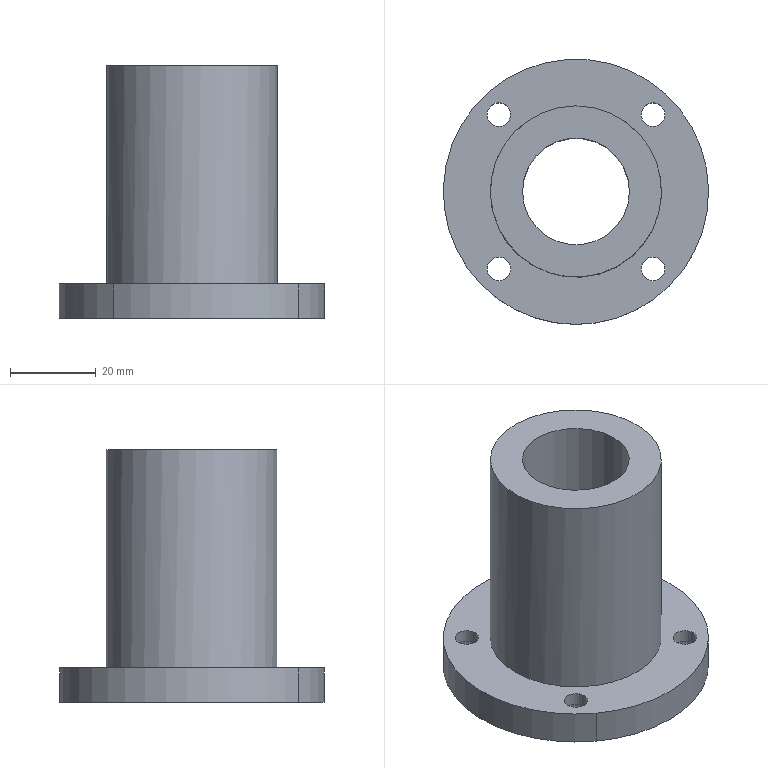Part | STEP file | YBQDJ-QD-7 | 1 solid | 19 faces | box 62 x 62 x 59 mm | volume 57722 mm3 | cylinder 12 | plane 7 | commonest cylinder face diameters 5.5 x4 9 x4 62 x2 25 x1 40 x1
STEP:
#1=CARTESIAN_POINT('',(0.,0.,0.));
#2=DIRECTION('',(0.,0.,1.));
#3=DIRECTION('',(1.,0.,0.));
#4=AXIS2_PLACEMENT_3D('',#1,#2,#3);
#5=CARTESIAN_POINT('',(-327.5,-310.,166.));
#6=VERTEX_POINT('',#5);
#7=CARTESIAN_POINT('',(-340.,-310.,166.));
#8=DIRECTION('',(0.,0.,-1.));
#9=DIRECTION('',(1.,0.,0.));
#10=AXIS2_PLACEMENT_3D('',#7,#8,#9);
#11=CIRCLE('',#10,12.5);
#12=CARTESIAN_POINT('',(-340.,-310.,166.));
#13=DIRECTION('',(0.,0.,-1.));
#14=DIRECTION('',(1.,0.,0.));
#15=AXIS2_PLACEMENT_3D('',#12,#13,#14);
#16=PLANE('',#15);
#17=CARTESIAN_POINT('',(0.,0.));
#18=DIRECTION('',(1.,0.));
#19=AXIS2_PLACEMENT_2D('',#17,#18);
#20=CIRCLE('',#19,12.5);
#21=(GEOMETRIC_REPRESENTATION_CONTEXT(2)PARAMETRIC_REPRESENTATION_CONTEXT()REPRESENTATION_CONTEXT('',''));
#22=DEFINITIONAL_REPRESENTATION('',(#20),#21);
#23=PCURVE('',#16,#22);
#24=CARTESIAN_POINT('',(-340.,-310.,225.));
#25=DIRECTION('',(0.,0.,-1.));
#26=DIRECTION('',(1.,0.,0.));
#27=AXIS2_PLACEMENT_3D('',#24,#25,#26);
#28=CYLINDRICAL_SURFACE('',#27,12.5);
#29=CARTESIAN_POINT('',(0.,59.));
#30=DIRECTION('',(1.,0.));
#31=VECTOR('',#30,1.);
#32=LINE('',#29,#31);
#33=(GEOMETRIC_REPRESENTATION_CONTEXT(2)PARAMETRIC_REPRESENTATION_CONTEXT()REPRESENTATION_CONTEXT('',''));
#34=DEFINITIONAL_REPRESENTATION('',(#32),#33);
#35=PCURVE('',#28,#34);
#36=SURFACE_CURVE('',#11,(#23,#35),.PCURVE_S1.);
#37=EDGE_CURVE('',#6,#6,#36,.T.);
#38=ORIENTED_EDGE('',*,*,#37,.F.);
#39=EDGE_LOOP('',(#38));
#40=FACE_BOUND('',#39,.T.);
#41=CARTESIAN_POINT('',(-326.469,-328.031,166.));
#42=VERTEX_POINT('',#41);
#43=CARTESIAN_POINT('',(-321.969,-328.031,166.));
#44=DIRECTION('',(0.,0.,1.));
#45=DIRECTION('',(-1.,0.,0.));
#46=AXIS2_PLACEMENT_3D('',#43,#44,#45);
#47=CIRCLE('',#46,4.5);
#48=CARTESIAN_POINT('',(13.531,18.031));
#49=CARTESIAN_POINT('',(13.531,25.825));
#50=CARTESIAN_POINT('',(20.281,21.928));
#51=CARTESIAN_POINT('',(27.031,18.031));
#52=CARTESIAN_POINT('',(20.281,14.134));
#53=CARTESIAN_POINT('',(13.531,10.237));
#54=CARTESIAN_POINT('',(13.531,18.031));
#55=(BOUNDED_CURVE()B_SPLINE_CURVE(2,(#48,#49,#50,#51,#52,#53,#54),.UNSPECIFIED.,.T.,.F.)B_SPLINE_CURVE_WITH_KNOTS((1,2,2,2,2,1),(-2.094,0.,2.094,4.189,6.283,8.378),.UNSPECIFIED.)CURVE()GEOMETRIC_REPRESENTATION_ITEM()RATIONAL_B_SPLINE_CURVE((1.,0.5,1.,0.5,1.,0.5,1.))REPRESENTATION_ITEM(''));
#56=(GEOMETRIC_REPRESENTATION_CONTEXT(2)PARAMETRIC_REPRESENTATION_CONTEXT()REPRESENTATION_CONTEXT('',''));
#57=DEFINITIONAL_REPRESENTATION('',(#55),#56);
#58=PCURVE('',#16,#57);
#59=CARTESIAN_POINT('',(-321.969,-328.031,166.));
#60=DIRECTION('',(0.,0.,1.));
#61=DIRECTION('',(-1.,0.,0.));
#62=AXIS2_PLACEMENT_3D('',#59,#60,#61);
#63=CYLINDRICAL_SURFACE('',#62,4.5);
#64=CARTESIAN_POINT('',(0.,0.));
#65=DIRECTION('',(1.,0.));
#66=VECTOR('',#65,1.);
#67=LINE('',#64,#66);
#68=(GEOMETRIC_REPRESENTATION_CONTEXT(2)PARAMETRIC_REPRESENTATION_CONTEXT()REPRESENTATION_CONTEXT('',''));
#69=DEFINITIONAL_REPRESENTATION('',(#67),#68);
#70=PCURVE('',#63,#69);
#71=SURFACE_CURVE('',#47,(#58,#70),.PCURVE_S1.);
#72=EDGE_CURVE('',#42,#42,#71,.T.);
#73=ORIENTED_EDGE('',*,*,#72,.T.);
#74=EDGE_LOOP('',(#73));
#75=FACE_BOUND('',#74,.T.);
#76=CARTESIAN_POINT('',(-362.531,-328.031,166.));
#77=VERTEX_POINT('',#76);
#78=CARTESIAN_POINT('',(-358.031,-328.031,166.));
#79=DIRECTION('',(0.,0.,1.));
#80=DIRECTION('',(-1.,0.,0.));
#81=AXIS2_PLACEMENT_3D('',#78,#79,#80);
#82=CIRCLE('',#81,4.5);
#83=CARTESIAN_POINT('',(-22.531,18.031));
#84=CARTESIAN_POINT('',(-22.531,25.825));
#85=CARTESIAN_POINT('',(-15.781,21.928));
#86=CARTESIAN_POINT('',(-9.031,18.031));
#87=CARTESIAN_POINT('',(-15.781,14.134));
#88=CARTESIAN_POINT('',(-22.531,10.237));
#89=CARTESIAN_POINT('',(-22.531,18.031));
#90=(BOUNDED_CURVE()B_SPLINE_CURVE(2,(#83,#84,#85,#86,#87,#88,#89),.UNSPECIFIED.,.T.,.F.)B_SPLINE_CURVE_WITH_KNOTS((1,2,2,2,2,1),(-2.094,0.,2.094,4.189,6.283,8.378),.UNSPECIFIED.)CURVE()GEOMETRIC_REPRESENTATION_ITEM()RATIONAL_B_SPLINE_CURVE((1.,0.5,1.,0.5,1.,0.5,1.))REPRESENTATION_ITEM(''));
#91=(GEOMETRIC_REPRESENTATION_CONTEXT(2)PARAMETRIC_REPRESENTATION_CONTEXT()REPRESENTATION_CONTEXT('',''));
#92=DEFINITIONAL_REPRESENTATION('',(#90),#91);
#93=PCURVE('',#16,#92);
#94=CARTESIAN_POINT('',(-358.031,-328.031,166.));
#95=DIRECTION('',(0.,0.,1.));
#96=DIRECTION('',(-1.,0.,0.));
#97=AXIS2_PLACEMENT_3D('',#94,#95,#96);
#98=CYLINDRICAL_SURFACE('',#97,4.5);
#99=CARTESIAN_POINT('',(0.,0.));
#100=DIRECTION('',(1.,0.));
#101=VECTOR('',#100,1.);
#102=LINE('',#99,#101);
#103=(GEOMETRIC_REPRESENTATION_CONTEXT(2)PARAMETRIC_REPRESENTATION_CONTEXT()REPRESENTATION_CONTEXT('',''));
#104=DEFINITIONAL_REPRESENTATION('',(#102),#103);
#105=PCURVE('',#98,#104);
#106=SURFACE_CURVE('',#82,(#93,#105),.PCURVE_S1.);
#107=EDGE_CURVE('',#77,#77,#106,.T.);
#108=ORIENTED_EDGE('',*,*,#107,.T.);
#109=EDGE_LOOP('',(#108));
#110=FACE_BOUND('',#109,.T.);
#111=CARTESIAN_POINT('',(-362.531,-291.969,166.));
#112=VERTEX_POINT('',#111);
#113=CARTESIAN_POINT('',(-358.031,-291.969,166.));
#114=DIRECTION('',(0.,0.,1.));
#115=DIRECTION('',(-1.,0.,0.));
#116=AXIS2_PLACEMENT_3D('',#113,#114,#115);
#117=CIRCLE('',#116,4.5);
#118=CARTESIAN_POINT('',(-22.531,-18.031));
#119=CARTESIAN_POINT('',(-22.531,-10.237));
#120=CARTESIAN_POINT('',(-15.781,-14.134));
#121=CARTESIAN_POINT('',(-9.031,-18.031));
#122=CARTESIAN_POINT('',(-15.781,-21.928));
#123=CARTESIAN_POINT('',(-22.531,-25.825));
#124=CARTESIAN_POINT('',(-22.531,-18.031));
#125=(BOUNDED_CURVE()B_SPLINE_CURVE(2,(#118,#119,#120,#121,#122,#123,#124),.UNSPECIFIED.,.T.,.F.)B_SPLINE_CURVE_WITH_KNOTS((1,2,2,2,2,1),(-2.094,0.,2.094,4.189,6.283,8.378),.UNSPECIFIED.)CURVE()GEOMETRIC_REPRESENTATION_ITEM()RATIONAL_B_SPLINE_CURVE((1.,0.5,1.,0.5,1.,0.5,1.))REPRESENTATION_ITEM(''));
#126=(GEOMETRIC_REPRESENTATION_CONTEXT(2)PARAMETRIC_REPRESENTATION_CONTEXT()REPRESENTATION_CONTEXT('',''));
#127=DEFINITIONAL_REPRESENTATION('',(#125),#126);
#128=PCURVE('',#16,#127);
#129=CARTESIAN_POINT('',(-358.031,-291.969,166.));
#130=DIRECTION('',(0.,0.,1.));
#131=DIRECTION('',(-1.,0.,0.));
#132=AXIS2_PLACEMENT_3D('',#129,#130,#131);
#133=CYLINDRICAL_SURFACE('',#132,4.5);
#134=CARTESIAN_POINT('',(0.,0.));
#135=DIRECTION('',(1.,0.));
#136=VECTOR('',#135,1.);
#137=LINE('',#134,#136);
#138=(GEOMETRIC_REPRESENTATION_CONTEXT(2)PARAMETRIC_REPRESENTATION_CONTEXT()REPRESENTATION_CONTEXT('',''));
#139=DEFINITIONAL_REPRESENTATION('',(#137),#138);
#140=PCURVE('',#133,#139);
#141=SURFACE_CURVE('',#117,(#128,#140),.PCURVE_S1.);
#142=EDGE_CURVE('',#112,#112,#141,.T.);
#143=ORIENTED_EDGE('',*,*,#142,.T.);
#144=EDGE_LOOP('',(#143));
#145=FACE_BOUND('',#144,.T.);
#146=CARTESIAN_POINT('',(-326.469,-291.969,166.));
#147=VERTEX_POINT('',#146);
#148=CARTESIAN_POINT('',(-321.969,-291.969,166.));
#149=DIRECTION('',(0.,0.,1.));
#150=DIRECTION('',(-1.,0.,0.));
#151=AXIS2_PLACEMENT_3D('',#148,#149,#150);
#152=CIRCLE('',#151,4.5);
#153=CARTESIAN_POINT('',(13.531,-18.031));
#154=CARTESIAN_POINT('',(13.531,-10.237));
#155=CARTESIAN_POINT('',(20.281,-14.134));
#156=CARTESIAN_POINT('',(27.031,-18.031));
#157=CARTESIAN_POINT('',(20.281,-21.928));
#158=CARTESIAN_POINT('',(13.531,-25.825));
#159=CARTESIAN_POINT('',(13.531,-18.031));
#160=(BOUNDED_CURVE()B_SPLINE_CURVE(2,(#153,#154,#155,#156,#157,#158,#159),.UNSPECIFIED.,.T.,.F.)B_SPLINE_CURVE_WITH_KNOTS((1,2,2,2,2,1),(-2.094,0.,2.094,4.189,6.283,8.378),.UNSPECIFIED.)CURVE()GEOMETRIC_REPRESENTATION_ITEM()RATIONAL_B_SPLINE_CURVE((1.,0.5,1.,0.5,1.,0.5,1.))REPRESENTATION_ITEM(''));
#161=(GEOMETRIC_REPRESENTATION_CONTEXT(2)PARAMETRIC_REPRESENTATION_CONTEXT()REPRESENTATION_CONTEXT('',''));
#162=DEFINITIONAL_REPRESENTATION('',(#160),#161);
#163=PCURVE('',#16,#162);
#164=CARTESIAN_POINT('',(-321.969,-291.969,166.));
#165=DIRECTION('',(0.,0.,1.));
#166=DIRECTION('',(-1.,0.,0.));
#167=AXIS2_PLACEMENT_3D('',#164,#165,#166);
#168=CYLINDRICAL_SURFACE('',#167,4.5);
#169=CARTESIAN_POINT('',(0.,0.));
#170=DIRECTION('',(1.,0.));
#171=VECTOR('',#170,1.);
#172=LINE('',#169,#171);
#173=(GEOMETRIC_REPRESENTATION_CONTEXT(2)PARAMETRIC_REPRESENTATION_CONTEXT()REPRESENTATION_CONTEXT('',''));
#174=DEFINITIONAL_REPRESENTATION('',(#172),#173);
#175=PCURVE('',#168,#174);
#176=SURFACE_CURVE('',#152,(#163,#175),.PCURVE_S1.);
#177=EDGE_CURVE('',#147,#147,#176,.T.);
#178=ORIENTED_EDGE('',*,*,#177,.T.);
#179=EDGE_LOOP('',(#178));
#180=FACE_BOUND('',#179,.T.);
#181=CARTESIAN_POINT('',(-315.,-328.33,166.));
#182=VERTEX_POINT('',#181);
#183=CARTESIAN_POINT('',(-358.33,-335.,166.));
#184=VERTEX_POINT('',#183);
#185=CARTESIAN_POINT('',(-340.,-310.,166.));
#186=DIRECTION('',(0.,0.,1.));
#187=DIRECTION('',(1.,0.,0.));
#188=AXIS2_PLACEMENT_3D('',#185,#186,#187);
#189=CIRCLE('',#188,31.);
#190=CARTESIAN_POINT('',(31.,0.));
#191=CARTESIAN_POINT('',(31.,-53.694));
#192=CARTESIAN_POINT('',(-15.5,-26.847));
#193=CARTESIAN_POINT('',(-62.,0.));
#194=CARTESIAN_POINT('',(-15.5,26.847));
#195=CARTESIAN_POINT('',(31.,53.694));
#196=CARTESIAN_POINT('',(31.,0.));
#197=(BOUNDED_CURVE()B_SPLINE_CURVE(2,(#190,#191,#192,#193,#194,#195,#196),.UNSPECIFIED.,.T.,.F.)B_SPLINE_CURVE_WITH_KNOTS((1,2,2,2,2,1),(-2.094,0.,2.094,4.189,6.283,8.378),.UNSPECIFIED.)CURVE()GEOMETRIC_REPRESENTATION_ITEM()RATIONAL_B_SPLINE_CURVE((1.,0.5,1.,0.5,1.,0.5,1.))REPRESENTATION_ITEM(''));
#198=(GEOMETRIC_REPRESENTATION_CONTEXT(2)PARAMETRIC_REPRESENTATION_CONTEXT()REPRESENTATION_CONTEXT('',''));
#199=DEFINITIONAL_REPRESENTATION('',(#197),#198);
#200=PCURVE('',#16,#199);
#201=CARTESIAN_POINT('',(-340.,-310.,174.));
#202=DIRECTION('',(0.,0.,-1.));
#203=DIRECTION('',(1.,0.,0.));
#204=AXIS2_PLACEMENT_3D('',#201,#202,#203);
#205=CYLINDRICAL_SURFACE('',#204,31.);
#206=CARTESIAN_POINT('',(12.566,8.));
#207=DIRECTION('',(-1.,0.));
#208=VECTOR('',#207,1.);
#209=LINE('',#206,#208);
#210=(GEOMETRIC_REPRESENTATION_CONTEXT(2)PARAMETRIC_REPRESENTATION_CONTEXT()REPRESENTATION_CONTEXT('',''));
#211=DEFINITIONAL_REPRESENTATION('',(#209),#210);
#212=PCURVE('',#205,#211);
#213=SURFACE_CURVE('',#189,(#200,#212),.PCURVE_S1.);
#214=EDGE_CURVE('',#182,#184,#213,.T.);
#215=ORIENTED_EDGE('',*,*,#214,.F.);
#216=CARTESIAN_POINT('',(-340.,-310.,166.));
#217=DIRECTION('',(0.,0.,1.));
#218=DIRECTION('',(1.,0.,0.));
#219=AXIS2_PLACEMENT_3D('',#216,#217,#218);
#220=CIRCLE('',#219,31.);
#221=CARTESIAN_POINT('',(31.,0.));
#222=CARTESIAN_POINT('',(31.,-53.694));
#223=CARTESIAN_POINT('',(-15.5,-26.847));
#224=CARTESIAN_POINT('',(-62.,0.));
#225=CARTESIAN_POINT('',(-15.5,26.847));
#226=CARTESIAN_POINT('',(31.,53.694));
#227=CARTESIAN_POINT('',(31.,0.));
#228=(BOUNDED_CURVE()B_SPLINE_CURVE(2,(#221,#222,#223,#224,#225,#226,#227),.UNSPECIFIED.,.T.,.F.)B_SPLINE_CURVE_WITH_KNOTS((1,2,2,2,2,1),(-2.094,0.,2.094,4.189,6.283,8.378),.UNSPECIFIED.)CURVE()GEOMETRIC_REPRESENTATION_ITEM()RATIONAL_B_SPLINE_CURVE((1.,0.5,1.,0.5,1.,0.5,1.))REPRESENTATION_ITEM(''));
#229=(GEOMETRIC_REPRESENTATION_CONTEXT(2)PARAMETRIC_REPRESENTATION_CONTEXT()REPRESENTATION_CONTEXT('',''));
#230=DEFINITIONAL_REPRESENTATION('',(#228),#229);
#231=PCURVE('',#16,#230);
#232=CARTESIAN_POINT('',(-340.,-310.,174.));
#233=DIRECTION('',(0.,0.,-1.));
#234=DIRECTION('',(1.,0.,0.));
#235=AXIS2_PLACEMENT_3D('',#232,#233,#234);
#236=CYLINDRICAL_SURFACE('',#235,31.);
#237=CARTESIAN_POINT('',(6.283,8.));
#238=DIRECTION('',(-1.,0.));
#239=VECTOR('',#238,1.);
#240=LINE('',#237,#239);
#241=(GEOMETRIC_REPRESENTATION_CONTEXT(2)PARAMETRIC_REPRESENTATION_CONTEXT()REPRESENTATION_CONTEXT('',''));
#242=DEFINITIONAL_REPRESENTATION('',(#240),#241);
#243=PCURVE('',#236,#242);
#244=SURFACE_CURVE('',#220,(#231,#243),.PCURVE_S1.);
#245=EDGE_CURVE('',#184,#182,#244,.T.);
#246=ORIENTED_EDGE('',*,*,#245,.F.);
#247=EDGE_LOOP('',(#215,#246));
#248=FACE_BOUND('',#247,.T.);
#249=ADVANCED_FACE('',(#40,#75,#110,#145,#180,#248),#16,.T.);
#250=CARTESIAN_POINT('',(-315.,-328.33,174.));
#251=VERTEX_POINT('',#250);
#252=CARTESIAN_POINT('',(-358.33,-335.,174.));
#253=VERTEX_POINT('',#252);
#254=CARTESIAN_POINT('',(-340.,-310.,174.));
#255=DIRECTION('',(0.,0.,1.));
#256=DIRECTION('',(-1.,0.,0.));
#257=AXIS2_PLACEMENT_3D('',#254,#255,#256);
#258=CIRCLE('',#257,31.);
#259=CARTESIAN_POINT('',(9.425,0.));
#260=DIRECTION('',(-1.,0.));
#261=VECTOR('',#260,1.);
#262=LINE('',#259,#261);
#263=(GEOMETRIC_REPRESENTATION_CONTEXT(2)PARAMETRIC_REPRESENTATION_CONTEXT()REPRESENTATION_CONTEXT('',''));
#264=DEFINITIONAL_REPRESENTATION('',(#262),#263);
#265=PCURVE('',#205,#264);
#266=CARTESIAN_POINT('',(92.5,-640.,174.));
#267=DIRECTION('',(0.,0.,1.));
#268=DIRECTION('',(-1.,0.,0.));
#269=AXIS2_PLACEMENT_3D('',#266,#267,#268);
#270=PLANE('',#269);
#271=CARTESIAN_POINT('',(432.5,-330.));
#272=DIRECTION('',(1.,0.));
#273=AXIS2_PLACEMENT_2D('',#271,#272);
#274=CIRCLE('',#273,31.);
#275=(GEOMETRIC_REPRESENTATION_CONTEXT(2)PARAMETRIC_REPRESENTATION_CONTEXT()REPRESENTATION_CONTEXT('',''));
#276=DEFINITIONAL_REPRESENTATION('',(#274),#275);
#277=PCURVE('',#270,#276);
#278=SURFACE_CURVE('',#258,(#265,#277),.PCURVE_S1.);
#279=EDGE_CURVE('',#251,#253,#278,.T.);
#280=ORIENTED_EDGE('',*,*,#279,.F.);
#281=CARTESIAN_POINT('',(-315.,-328.33,170.));
#282=DIRECTION('',(0.,0.,1.));
#283=VECTOR('',#282,1.);
#284=LINE('',#281,#283);
#285=CARTESIAN_POINT('',(6.916,4.));
#286=DIRECTION('',(0.,-1.));
#287=VECTOR('',#286,1.);
#288=LINE('',#285,#287);
#289=(GEOMETRIC_REPRESENTATION_CONTEXT(2)PARAMETRIC_REPRESENTATION_CONTEXT()REPRESENTATION_CONTEXT('',''));
#290=DEFINITIONAL_REPRESENTATION('',(#288),#289);
#291=PCURVE('',#205,#290);
#292=CARTESIAN_POINT('',(0.6327,4.));
#293=DIRECTION('',(0.,-1.));
#294=VECTOR('',#293,1.);
#295=LINE('',#292,#294);
#296=(GEOMETRIC_REPRESENTATION_CONTEXT(2)PARAMETRIC_REPRESENTATION_CONTEXT()REPRESENTATION_CONTEXT('',''));
#297=DEFINITIONAL_REPRESENTATION('',(#295),#296);
#298=PCURVE('',#236,#297);
#299=SURFACE_CURVE('',#284,(#291,#298),.PCURVE_S1.);
#300=EDGE_CURVE('',#182,#251,#299,.T.);
#301=ORIENTED_EDGE('',*,*,#300,.F.);
#302=ORIENTED_EDGE('',*,*,#214,.T.);
#303=CARTESIAN_POINT('',(-358.33,-335.,170.));
#304=DIRECTION('',(0.,0.,-1.));
#305=VECTOR('',#304,1.);
#306=LINE('',#303,#305);
#307=CARTESIAN_POINT('',(2.203,4.));
#308=DIRECTION('',(0.,1.));
#309=VECTOR('',#308,1.);
#310=LINE('',#307,#309);
#311=(GEOMETRIC_REPRESENTATION_CONTEXT(2)PARAMETRIC_REPRESENTATION_CONTEXT()REPRESENTATION_CONTEXT('',''));
#312=DEFINITIONAL_REPRESENTATION('',(#310),#311);
#313=PCURVE('',#205,#312);
#314=CARTESIAN_POINT('',(2.203,4.));
#315=DIRECTION('',(0.,1.));
#316=VECTOR('',#315,1.);
#317=LINE('',#314,#316);
#318=(GEOMETRIC_REPRESENTATION_CONTEXT(2)PARAMETRIC_REPRESENTATION_CONTEXT()REPRESENTATION_CONTEXT('',''));
#319=DEFINITIONAL_REPRESENTATION('',(#317),#318);
#320=PCURVE('',#236,#319);
#321=SURFACE_CURVE('',#306,(#313,#320),.PCURVE_S1.);
#322=EDGE_CURVE('',#253,#184,#321,.T.);
#323=ORIENTED_EDGE('',*,*,#322,.F.);
#324=EDGE_LOOP('',(#280,#301,#302,#323));
#325=FACE_BOUND('',#324,.T.);
#326=ADVANCED_FACE('',(#325),#205,.T.);
#327=ORIENTED_EDGE('',*,*,#245,.T.);
#328=ORIENTED_EDGE('',*,*,#300,.T.);
#329=CARTESIAN_POINT('',(-340.,-310.,174.));
#330=DIRECTION('',(0.,0.,1.));
#331=DIRECTION('',(-1.,0.,0.));
#332=AXIS2_PLACEMENT_3D('',#329,#330,#331);
#333=CIRCLE('',#332,31.);
#334=CARTESIAN_POINT('',(3.142,0.));
#335=DIRECTION('',(-1.,0.));
#336=VECTOR('',#335,1.);
#337=LINE('',#334,#336);
#338=(GEOMETRIC_REPRESENTATION_CONTEXT(2)PARAMETRIC_REPRESENTATION_CONTEXT()REPRESENTATION_CONTEXT('',''));
#339=DEFINITIONAL_REPRESENTATION('',(#337),#338);
#340=PCURVE('',#236,#339);
#341=CARTESIAN_POINT('',(432.5,-330.));
#342=DIRECTION('',(1.,0.));
#343=AXIS2_PLACEMENT_2D('',#341,#342);
#344=CIRCLE('',#343,31.);
#345=(GEOMETRIC_REPRESENTATION_CONTEXT(2)PARAMETRIC_REPRESENTATION_CONTEXT()REPRESENTATION_CONTEXT('',''));
#346=DEFINITIONAL_REPRESENTATION('',(#344),#345);
#347=PCURVE('',#270,#346);
#348=SURFACE_CURVE('',#333,(#340,#347),.PCURVE_S1.);
#349=EDGE_CURVE('',#253,#251,#348,.T.);
#350=ORIENTED_EDGE('',*,*,#349,.F.);
#351=ORIENTED_EDGE('',*,*,#322,.T.);
#352=EDGE_LOOP('',(#327,#328,#350,#351));
#353=FACE_BOUND('',#352,.T.);
#354=ADVANCED_FACE('',(#353),#236,.T.);
#355=CARTESIAN_POINT('',(-360.,-310.,174.));
#356=VERTEX_POINT('',#355);
#357=CARTESIAN_POINT('',(-340.,-290.,174.));
#358=VERTEX_POINT('',#357);
#359=CARTESIAN_POINT('',(-340.,-310.,174.));
#360=DIRECTION('',(0.,0.,-1.));
#361=DIRECTION('',(-1.,0.,0.));
#362=AXIS2_PLACEMENT_3D('',#359,#360,#361);
#363=CIRCLE('',#362,20.);
#364=CARTESIAN_POINT('',(452.5,-330.));
#365=CARTESIAN_POINT('',(452.5,-364.641));
#366=CARTESIAN_POINT('',(422.5,-347.321));
#367=CARTESIAN_POINT('',(392.5,-330.));
#368=CARTESIAN_POINT('',(422.5,-312.679));
#369=CARTESIAN_POINT('',(452.5,-295.359));
#370=CARTESIAN_POINT('',(452.5,-330.));
#371=(BOUNDED_CURVE()B_SPLINE_CURVE(2,(#364,#365,#366,#367,#368,#369,#370),.UNSPECIFIED.,.T.,.F.)B_SPLINE_CURVE_WITH_KNOTS((1,2,2,2,2,1),(-2.094,0.,2.094,4.189,6.283,8.378),.UNSPECIFIED.)CURVE()GEOMETRIC_REPRESENTATION_ITEM()RATIONAL_B_SPLINE_CURVE((1.,0.5,1.,0.5,1.,0.5,1.))REPRESENTATION_ITEM(''));
#372=(GEOMETRIC_REPRESENTATION_CONTEXT(2)PARAMETRIC_REPRESENTATION_CONTEXT()REPRESENTATION_CONTEXT('',''));
#373=DEFINITIONAL_REPRESENTATION('',(#371),#372);
#374=PCURVE('',#270,#373);
#375=CARTESIAN_POINT('',(-340.,-310.,225.));
#376=DIRECTION('',(0.,0.,-1.));
#377=DIRECTION('',(1.,0.,0.));
#378=AXIS2_PLACEMENT_3D('',#375,#376,#377);
#379=CYLINDRICAL_SURFACE('',#378,20.);
#380=CARTESIAN_POINT('',(9.425,51.));
#381=DIRECTION('',(1.,0.));
#382=VECTOR('',#381,1.);
#383=LINE('',#380,#382);
#384=(GEOMETRIC_REPRESENTATION_CONTEXT(2)PARAMETRIC_REPRESENTATION_CONTEXT()REPRESENTATION_CONTEXT('',''));
#385=DEFINITIONAL_REPRESENTATION('',(#383),#384);
#386=PCURVE('',#379,#385);
#387=SURFACE_CURVE('',#363,(#374,#386),.PCURVE_S1.);
#388=EDGE_CURVE('',#356,#358,#387,.T.);
#389=ORIENTED_EDGE('',*,*,#388,.T.);
#390=CARTESIAN_POINT('',(-340.,-310.,174.));
#391=DIRECTION('',(0.,0.,-1.));
#392=DIRECTION('',(-1.,0.,0.));
#393=AXIS2_PLACEMENT_3D('',#390,#391,#392);
#394=CIRCLE('',#393,20.);
#395=CARTESIAN_POINT('',(452.5,-330.));
#396=CARTESIAN_POINT('',(452.5,-364.641));
#397=CARTESIAN_POINT('',(422.5,-347.321));
#398=CARTESIAN_POINT('',(392.5,-330.));
#399=CARTESIAN_POINT('',(422.5,-312.679));
#400=CARTESIAN_POINT('',(452.5,-295.359));
#401=CARTESIAN_POINT('',(452.5,-330.));
#402=(BOUNDED_CURVE()B_SPLINE_CURVE(2,(#395,#396,#397,#398,#399,#400,#401),.UNSPECIFIED.,.T.,.F.)B_SPLINE_CURVE_WITH_KNOTS((1,2,2,2,2,1),(-2.094,0.,2.094,4.189,6.283,8.378),.UNSPECIFIED.)CURVE()GEOMETRIC_REPRESENTATION_ITEM()RATIONAL_B_SPLINE_CURVE((1.,0.5,1.,0.5,1.,0.5,1.))REPRESENTATION_ITEM(''));
#403=(GEOMETRIC_REPRESENTATION_CONTEXT(2)PARAMETRIC_REPRESENTATION_CONTEXT()REPRESENTATION_CONTEXT('',''));
#404=DEFINITIONAL_REPRESENTATION('',(#402),#403);
#405=PCURVE('',#270,#404);
#406=CARTESIAN_POINT('',(3.142,51.));
#407=DIRECTION('',(1.,0.));
#408=VECTOR('',#407,1.);
#409=LINE('',#406,#408);
#410=(GEOMETRIC_REPRESENTATION_CONTEXT(2)PARAMETRIC_REPRESENTATION_CONTEXT()REPRESENTATION_CONTEXT('',''));
#411=DEFINITIONAL_REPRESENTATION('',(#409),#410);
#412=PCURVE('',#379,#411);
#413=SURFACE_CURVE('',#394,(#405,#412),.PCURVE_S1.);
#414=EDGE_CURVE('',#358,#356,#413,.T.);
#415=ORIENTED_EDGE('',*,*,#414,.T.);
#416=EDGE_LOOP('',(#389,#415));
#417=FACE_BOUND('',#416,.T.);
#418=CARTESIAN_POINT('',(-324.719,-328.031,174.));
#419=VERTEX_POINT('',#418);
#420=CARTESIAN_POINT('',(-321.969,-328.031,174.));
#421=DIRECTION('',(0.,0.,1.));
#422=DIRECTION('',(-1.,0.,0.));
#423=AXIS2_PLACEMENT_3D('',#420,#421,#422);
#424=CIRCLE('',#423,2.75);
#425=CARTESIAN_POINT('',(414.469,-311.969));
#426=DIRECTION('',(1.,0.));
#427=AXIS2_PLACEMENT_2D('',#425,#426);
#428=CIRCLE('',#427,2.75);
#429=(GEOMETRIC_REPRESENTATION_CONTEXT(2)PARAMETRIC_REPRESENTATION_CONTEXT()REPRESENTATION_CONTEXT('',''));
#430=DEFINITIONAL_REPRESENTATION('',(#428),#429);
#431=PCURVE('',#270,#430);
#432=CARTESIAN_POINT('',(-321.969,-328.031,216.));
#433=DIRECTION('',(0.,0.,1.));
#434=DIRECTION('',(-1.,0.,0.));
#435=AXIS2_PLACEMENT_3D('',#432,#433,#434);
#436=CYLINDRICAL_SURFACE('',#435,2.75);
#437=CARTESIAN_POINT('',(0.,-42.));
#438=DIRECTION('',(1.,0.));
#439=VECTOR('',#438,1.);
#440=LINE('',#437,#439);
#441=(GEOMETRIC_REPRESENTATION_CONTEXT(2)PARAMETRIC_REPRESENTATION_CONTEXT()REPRESENTATION_CONTEXT('',''));
#442=DEFINITIONAL_REPRESENTATION('',(#440),#441);
#443=PCURVE('',#436,#442);
#444=SURFACE_CURVE('',#424,(#431,#443),.PCURVE_S1.);
#445=EDGE_CURVE('',#419,#419,#444,.T.);
#446=ORIENTED_EDGE('',*,*,#445,.F.);
#447=EDGE_LOOP('',(#446));
#448=FACE_BOUND('',#447,.T.);
#449=CARTESIAN_POINT('',(-360.781,-328.031,174.));
#450=VERTEX_POINT('',#449);
#451=CARTESIAN_POINT('',(-358.031,-328.031,174.));
#452=DIRECTION('',(0.,0.,1.));
#453=DIRECTION('',(-1.,0.,0.));
#454=AXIS2_PLACEMENT_3D('',#451,#452,#453);
#455=CIRCLE('',#454,2.75);
#456=CARTESIAN_POINT('',(450.531,-311.969));
#457=DIRECTION('',(1.,0.));
#458=AXIS2_PLACEMENT_2D('',#456,#457);
#459=CIRCLE('',#458,2.75);
#460=(GEOMETRIC_REPRESENTATION_CONTEXT(2)PARAMETRIC_REPRESENTATION_CONTEXT()REPRESENTATION_CONTEXT('',''));
#461=DEFINITIONAL_REPRESENTATION('',(#459),#460);
#462=PCURVE('',#270,#461);
#463=CARTESIAN_POINT('',(-358.031,-328.031,216.));
#464=DIRECTION('',(0.,0.,1.));
#465=DIRECTION('',(-1.,0.,0.));
#466=AXIS2_PLACEMENT_3D('',#463,#464,#465);
#467=CYLINDRICAL_SURFACE('',#466,2.75);
#468=CARTESIAN_POINT('',(0.,-42.));
#469=DIRECTION('',(1.,0.));
#470=VECTOR('',#469,1.);
#471=LINE('',#468,#470);
#472=(GEOMETRIC_REPRESENTATION_CONTEXT(2)PARAMETRIC_REPRESENTATION_CONTEXT()REPRESENTATION_CONTEXT('',''));
#473=DEFINITIONAL_REPRESENTATION('',(#471),#472);
#474=PCURVE('',#467,#473);
#475=SURFACE_CURVE('',#455,(#462,#474),.PCURVE_S1.);
#476=EDGE_CURVE('',#450,#450,#475,.T.);
#477=ORIENTED_EDGE('',*,*,#476,.F.);
#478=EDGE_LOOP('',(#477));
#479=FACE_BOUND('',#478,.T.);
#480=CARTESIAN_POINT('',(-360.781,-291.969,174.));
#481=VERTEX_POINT('',#480);
#482=CARTESIAN_POINT('',(-358.031,-291.969,174.));
#483=DIRECTION('',(0.,0.,1.));
#484=DIRECTION('',(-1.,0.,0.));
#485=AXIS2_PLACEMENT_3D('',#482,#483,#484);
#486=CIRCLE('',#485,2.75);
#487=CARTESIAN_POINT('',(450.531,-348.031));
#488=DIRECTION('',(1.,0.));
#489=AXIS2_PLACEMENT_2D('',#487,#488);
#490=CIRCLE('',#489,2.75);
#491=(GEOMETRIC_REPRESENTATION_CONTEXT(2)PARAMETRIC_REPRESENTATION_CONTEXT()REPRESENTATION_CONTEXT('',''));
#492=DEFINITIONAL_REPRESENTATION('',(#490),#491);
#493=PCURVE('',#270,#492);
#494=CARTESIAN_POINT('',(-358.031,-291.969,216.));
#495=DIRECTION('',(0.,0.,1.));
#496=DIRECTION('',(-1.,0.,0.));
#497=AXIS2_PLACEMENT_3D('',#494,#495,#496);
#498=CYLINDRICAL_SURFACE('',#497,2.75);
#499=CARTESIAN_POINT('',(0.,-42.));
#500=DIRECTION('',(1.,0.));
#501=VECTOR('',#500,1.);
#502=LINE('',#499,#501);
#503=(GEOMETRIC_REPRESENTATION_CONTEXT(2)PARAMETRIC_REPRESENTATION_CONTEXT()REPRESENTATION_CONTEXT('',''));
#504=DEFINITIONAL_REPRESENTATION('',(#502),#503);
#505=PCURVE('',#498,#504);
#506=SURFACE_CURVE('',#486,(#493,#505),.PCURVE_S1.);
#507=EDGE_CURVE('',#481,#481,#506,.T.);
#508=ORIENTED_EDGE('',*,*,#507,.F.);
#509=EDGE_LOOP('',(#508));
#510=FACE_BOUND('',#509,.T.);
#511=CARTESIAN_POINT('',(-324.719,-291.969,174.));
#512=VERTEX_POINT('',#511);
#513=CARTESIAN_POINT('',(-321.969,-291.969,174.));
#514=DIRECTION('',(0.,0.,1.));
#515=DIRECTION('',(-1.,0.,0.));
#516=AXIS2_PLACEMENT_3D('',#513,#514,#515);
#517=CIRCLE('',#516,2.75);
#518=CARTESIAN_POINT('',(414.469,-348.031));
#519=DIRECTION('',(1.,0.));
#520=AXIS2_PLACEMENT_2D('',#518,#519);
#521=CIRCLE('',#520,2.75);
#522=(GEOMETRIC_REPRESENTATION_CONTEXT(2)PARAMETRIC_REPRESENTATION_CONTEXT()REPRESENTATION_CONTEXT('',''));
#523=DEFINITIONAL_REPRESENTATION('',(#521),#522);
#524=PCURVE('',#270,#523);
#525=CARTESIAN_POINT('',(-321.969,-291.969,216.));
#526=DIRECTION('',(0.,0.,1.));
#527=DIRECTION('',(-1.,0.,0.));
#528=AXIS2_PLACEMENT_3D('',#525,#526,#527);
#529=CYLINDRICAL_SURFACE('',#528,2.75);
#530=CARTESIAN_POINT('',(0.,-42.));
#531=DIRECTION('',(1.,0.));
#532=VECTOR('',#531,1.);
#533=LINE('',#530,#532);
#534=(GEOMETRIC_REPRESENTATION_CONTEXT(2)PARAMETRIC_REPRESENTATION_CONTEXT()REPRESENTATION_CONTEXT('',''));
#535=DEFINITIONAL_REPRESENTATION('',(#533),#534);
#536=PCURVE('',#529,#535);
#537=SURFACE_CURVE('',#517,(#524,#536),.PCURVE_S1.);
#538=EDGE_CURVE('',#512,#512,#537,.T.);
#539=ORIENTED_EDGE('',*,*,#538,.F.);
#540=EDGE_LOOP('',(#539));
#541=FACE_BOUND('',#540,.T.);
#542=ORIENTED_EDGE('',*,*,#349,.T.);
#543=ORIENTED_EDGE('',*,*,#279,.T.);
#544=EDGE_LOOP('',(#542,#543));
#545=FACE_BOUND('',#544,.T.);
#546=ADVANCED_FACE('',(#417,#448,#479,#510,#541,#545),#270,.T.);
#547=ORIENTED_EDGE('',*,*,#538,.F.);
#548=CARTESIAN_POINT('',(-324.719,-291.969,171.));
#549=VERTEX_POINT('',#548);
#550=CARTESIAN_POINT('',(-324.719,-291.969,171.));
#551=CARTESIAN_POINT('',(-324.719,-291.969,174.));
#552=B_SPLINE_CURVE_WITH_KNOTS('',1,(#550,#551),.UNSPECIFIED.,.F.,.F.,(2,2),(-45.,-42.),.PIECEWISE_BEZIER_KNOTS.);
#553=CARTESIAN_POINT('',(0.,0.));
#554=DIRECTION('',(0.,1.));
#555=VECTOR('',#554,1.);
#556=LINE('',#553,#555);
#557=(GEOMETRIC_REPRESENTATION_CONTEXT(2)PARAMETRIC_REPRESENTATION_CONTEXT()REPRESENTATION_CONTEXT('',''));
#558=DEFINITIONAL_REPRESENTATION('',(#556),#557);
#559=PCURVE('',#529,#558);
#560=CARTESIAN_POINT('',(6.283,0.));
#561=DIRECTION('',(0.,1.));
#562=VECTOR('',#561,1.);
#563=LINE('',#560,#562);
#564=(GEOMETRIC_REPRESENTATION_CONTEXT(2)PARAMETRIC_REPRESENTATION_CONTEXT()REPRESENTATION_CONTEXT('',''));
#565=DEFINITIONAL_REPRESENTATION('',(#563),#564);
#566=PCURVE('',#529,#565);
#567=SEAM_CURVE('',#552,(#559,#566),.PCURVE_S1.);
#568=EDGE_CURVE('',#549,#512,#567,.T.);
#569=ORIENTED_EDGE('',*,*,#568,.F.);
#570=CARTESIAN_POINT('',(-321.969,-291.969,171.));
#571=DIRECTION('',(0.,0.,-1.));
#572=DIRECTION('',(-1.,0.,0.));
#573=AXIS2_PLACEMENT_3D('',#570,#571,#572);
#574=CIRCLE('',#573,2.75);
#575=CARTESIAN_POINT('',(6.283,-45.));
#576=DIRECTION('',(-1.,0.));
#577=VECTOR('',#576,1.);
#578=LINE('',#575,#577);
#579=(GEOMETRIC_REPRESENTATION_CONTEXT(2)PARAMETRIC_REPRESENTATION_CONTEXT()REPRESENTATION_CONTEXT('',''));
#580=DEFINITIONAL_REPRESENTATION('',(#578),#579);
#581=PCURVE('',#529,#580);
#582=CARTESIAN_POINT('',(-321.969,-291.969,171.));
#583=DIRECTION('',(0.,0.,1.));
#584=DIRECTION('',(-1.,0.,0.));
#585=AXIS2_PLACEMENT_3D('',#582,#583,#584);
#586=PLANE('',#585);
#587=CARTESIAN_POINT('',(2.75,0.));
#588=CARTESIAN_POINT('',(2.75,-4.763));
#589=CARTESIAN_POINT('',(-1.375,-2.382));
#590=CARTESIAN_POINT('',(-5.5,0.));
#591=CARTESIAN_POINT('',(-1.375,2.382));
#592=CARTESIAN_POINT('',(2.75,4.763));
#593=CARTESIAN_POINT('',(2.75,0.));
#594=(BOUNDED_CURVE()B_SPLINE_CURVE(2,(#587,#588,#589,#590,#591,#592,#593),.UNSPECIFIED.,.T.,.F.)B_SPLINE_CURVE_WITH_KNOTS((1,2,2,2,2,1),(-2.094,0.,2.094,4.189,6.283,8.378),.UNSPECIFIED.)CURVE()GEOMETRIC_REPRESENTATION_ITEM()RATIONAL_B_SPLINE_CURVE((1.,0.5,1.,0.5,1.,0.5,1.))REPRESENTATION_ITEM(''));
#595=(GEOMETRIC_REPRESENTATION_CONTEXT(2)PARAMETRIC_REPRESENTATION_CONTEXT()REPRESENTATION_CONTEXT('',''));
#596=DEFINITIONAL_REPRESENTATION('',(#594),#595);
#597=PCURVE('',#586,#596);
#598=SURFACE_CURVE('',#574,(#581,#597),.PCURVE_S1.);
#599=EDGE_CURVE('',#549,#549,#598,.T.);
#600=ORIENTED_EDGE('',*,*,#599,.F.);
#601=ORIENTED_EDGE('',*,*,#568,.T.);
#602=EDGE_LOOP('',(#547,#569,#600,#601));
#603=FACE_BOUND('',#602,.F.);
#604=ADVANCED_FACE('',(#603),#529,.F.);
#605=ORIENTED_EDGE('',*,*,#599,.F.);
#606=EDGE_LOOP('',(#605));
#607=FACE_BOUND('',#606,.T.);
#608=CARTESIAN_POINT('',(-326.469,-291.969,171.));
#609=VERTEX_POINT('',#608);
#610=CARTESIAN_POINT('',(-321.969,-291.969,171.));
#611=DIRECTION('',(0.,0.,-1.));
#612=DIRECTION('',(-1.,0.,0.));
#613=AXIS2_PLACEMENT_3D('',#610,#611,#612);
#614=CIRCLE('',#613,4.5);
#615=CARTESIAN_POINT('',(4.5,0.));
#616=CARTESIAN_POINT('',(4.5,-7.794));
#617=CARTESIAN_POINT('',(-2.25,-3.897));
#618=CARTESIAN_POINT('',(-9.,0.));
#619=CARTESIAN_POINT('',(-2.25,3.897));
#620=CARTESIAN_POINT('',(4.5,7.794));
#621=CARTESIAN_POINT('',(4.5,0.));
#622=(BOUNDED_CURVE()B_SPLINE_CURVE(2,(#615,#616,#617,#618,#619,#620,#621),.UNSPECIFIED.,.T.,.F.)B_SPLINE_CURVE_WITH_KNOTS((1,2,2,2,2,1),(-2.094,0.,2.094,4.189,6.283,8.378),.UNSPECIFIED.)CURVE()GEOMETRIC_REPRESENTATION_ITEM()RATIONAL_B_SPLINE_CURVE((1.,0.5,1.,0.5,1.,0.5,1.))REPRESENTATION_ITEM(''));
#623=(GEOMETRIC_REPRESENTATION_CONTEXT(2)PARAMETRIC_REPRESENTATION_CONTEXT()REPRESENTATION_CONTEXT('',''));
#624=DEFINITIONAL_REPRESENTATION('',(#622),#623);
#625=PCURVE('',#586,#624);
#626=CARTESIAN_POINT('',(6.283,5.));
#627=DIRECTION('',(-1.,0.));
#628=VECTOR('',#627,1.);
#629=LINE('',#626,#628);
#630=(GEOMETRIC_REPRESENTATION_CONTEXT(2)PARAMETRIC_REPRESENTATION_CONTEXT()REPRESENTATION_CONTEXT('',''));
#631=DEFINITIONAL_REPRESENTATION('',(#629),#630);
#632=PCURVE('',#168,#631);
#633=SURFACE_CURVE('',#614,(#625,#632),.PCURVE_S1.);
#634=EDGE_CURVE('',#609,#609,#633,.T.);
#635=ORIENTED_EDGE('',*,*,#634,.T.);
#636=EDGE_LOOP('',(#635));
#637=FACE_BOUND('',#636,.T.);
#638=ADVANCED_FACE('',(#607,#637),#586,.F.);
#639=ORIENTED_EDGE('',*,*,#634,.T.);
#640=CARTESIAN_POINT('',(-326.469,-291.969,166.));
#641=CARTESIAN_POINT('',(-326.469,-291.969,171.));
#642=B_SPLINE_CURVE_WITH_KNOTS('',1,(#640,#641),.UNSPECIFIED.,.F.,.F.,(2,2),(0.,5.),.PIECEWISE_BEZIER_KNOTS.);
#643=CARTESIAN_POINT('',(0.,0.));
#644=DIRECTION('',(0.,1.));
#645=VECTOR('',#644,1.);
#646=LINE('',#643,#645);
#647=(GEOMETRIC_REPRESENTATION_CONTEXT(2)PARAMETRIC_REPRESENTATION_CONTEXT()REPRESENTATION_CONTEXT('',''));
#648=DEFINITIONAL_REPRESENTATION('',(#646),#647);
#649=PCURVE('',#168,#648);
#650=CARTESIAN_POINT('',(6.283,0.));
#651=DIRECTION('',(0.,1.));
#652=VECTOR('',#651,1.);
#653=LINE('',#650,#652);
#654=(GEOMETRIC_REPRESENTATION_CONTEXT(2)PARAMETRIC_REPRESENTATION_CONTEXT()REPRESENTATION_CONTEXT('',''));
#655=DEFINITIONAL_REPRESENTATION('',(#653),#654);
#656=PCURVE('',#168,#655);
#657=SEAM_CURVE('',#642,(#649,#656),.PCURVE_S1.);
#658=EDGE_CURVE('',#147,#609,#657,.T.);
#659=ORIENTED_EDGE('',*,*,#658,.F.);
#660=ORIENTED_EDGE('',*,*,#177,.T.);
#661=ORIENTED_EDGE('',*,*,#658,.T.);
#662=EDGE_LOOP('',(#639,#659,#660,#661));
#663=FACE_BOUND('',#662,.F.);
#664=ADVANCED_FACE('',(#663),#168,.F.);
#665=ORIENTED_EDGE('',*,*,#507,.F.);
#666=CARTESIAN_POINT('',(-360.781,-291.969,171.));
#667=VERTEX_POINT('',#666);
#668=CARTESIAN_POINT('',(-360.781,-291.969,171.));
#669=CARTESIAN_POINT('',(-360.781,-291.969,174.));
#670=B_SPLINE_CURVE_WITH_KNOTS('',1,(#668,#669),.UNSPECIFIED.,.F.,.F.,(2,2),(-45.,-42.),.PIECEWISE_BEZIER_KNOTS.);
#671=CARTESIAN_POINT('',(0.,0.));
#672=DIRECTION('',(0.,1.));
#673=VECTOR('',#672,1.);
#674=LINE('',#671,#673);
#675=(GEOMETRIC_REPRESENTATION_CONTEXT(2)PARAMETRIC_REPRESENTATION_CONTEXT()REPRESENTATION_CONTEXT('',''));
#676=DEFINITIONAL_REPRESENTATION('',(#674),#675);
#677=PCURVE('',#498,#676);
#678=CARTESIAN_POINT('',(6.283,0.));
#679=DIRECTION('',(0.,1.));
#680=VECTOR('',#679,1.);
#681=LINE('',#678,#680);
#682=(GEOMETRIC_REPRESENTATION_CONTEXT(2)PARAMETRIC_REPRESENTATION_CONTEXT()REPRESENTATION_CONTEXT('',''));
#683=DEFINITIONAL_REPRESENTATION('',(#681),#682);
#684=PCURVE('',#498,#683);
#685=SEAM_CURVE('',#670,(#677,#684),.PCURVE_S1.);
#686=EDGE_CURVE('',#667,#481,#685,.T.);
#687=ORIENTED_EDGE('',*,*,#686,.F.);
#688=CARTESIAN_POINT('',(-358.031,-291.969,171.));
#689=DIRECTION('',(0.,0.,-1.));
#690=DIRECTION('',(-1.,0.,0.));
#691=AXIS2_PLACEMENT_3D('',#688,#689,#690);
#692=CIRCLE('',#691,2.75);
#693=CARTESIAN_POINT('',(6.283,-45.));
#694=DIRECTION('',(-1.,0.));
#695=VECTOR('',#694,1.);
#696=LINE('',#693,#695);
#697=(GEOMETRIC_REPRESENTATION_CONTEXT(2)PARAMETRIC_REPRESENTATION_CONTEXT()REPRESENTATION_CONTEXT('',''));
#698=DEFINITIONAL_REPRESENTATION('',(#696),#697);
#699=PCURVE('',#498,#698);
#700=CARTESIAN_POINT('',(-358.031,-291.969,171.));
#701=DIRECTION('',(0.,0.,1.));
#702=DIRECTION('',(-1.,0.,0.));
#703=AXIS2_PLACEMENT_3D('',#700,#701,#702);
#704=PLANE('',#703);
#705=CARTESIAN_POINT('',(2.75,0.));
#706=CARTESIAN_POINT('',(2.75,-4.763));
#707=CARTESIAN_POINT('',(-1.375,-2.382));
#708=CARTESIAN_POINT('',(-5.5,0.));
#709=CARTESIAN_POINT('',(-1.375,2.382));
#710=CARTESIAN_POINT('',(2.75,4.763));
#711=CARTESIAN_POINT('',(2.75,0.));
#712=(BOUNDED_CURVE()B_SPLINE_CURVE(2,(#705,#706,#707,#708,#709,#710,#711),.UNSPECIFIED.,.T.,.F.)B_SPLINE_CURVE_WITH_KNOTS((1,2,2,2,2,1),(-2.094,0.,2.094,4.189,6.283,8.378),.UNSPECIFIED.)CURVE()GEOMETRIC_REPRESENTATION_ITEM()RATIONAL_B_SPLINE_CURVE((1.,0.5,1.,0.5,1.,0.5,1.))REPRESENTATION_ITEM(''));
#713=(GEOMETRIC_REPRESENTATION_CONTEXT(2)PARAMETRIC_REPRESENTATION_CONTEXT()REPRESENTATION_CONTEXT('',''));
#714=DEFINITIONAL_REPRESENTATION('',(#712),#713);
#715=PCURVE('',#704,#714);
#716=SURFACE_CURVE('',#692,(#699,#715),.PCURVE_S1.);
#717=EDGE_CURVE('',#667,#667,#716,.T.);
#718=ORIENTED_EDGE('',*,*,#717,.F.);
#719=ORIENTED_EDGE('',*,*,#686,.T.);
#720=EDGE_LOOP('',(#665,#687,#718,#719));
#721=FACE_BOUND('',#720,.F.);
#722=ADVANCED_FACE('',(#721),#498,.F.);
#723=ORIENTED_EDGE('',*,*,#717,.F.);
#724=EDGE_LOOP('',(#723));
#725=FACE_BOUND('',#724,.T.);
#726=CARTESIAN_POINT('',(-362.531,-291.969,171.));
#727=VERTEX_POINT('',#726);
#728=CARTESIAN_POINT('',(-358.031,-291.969,171.));
#729=DIRECTION('',(0.,0.,-1.));
#730=DIRECTION('',(-1.,0.,0.));
#731=AXIS2_PLACEMENT_3D('',#728,#729,#730);
#732=CIRCLE('',#731,4.5);
#733=CARTESIAN_POINT('',(4.5,0.));
#734=CARTESIAN_POINT('',(4.5,-7.794));
#735=CARTESIAN_POINT('',(-2.25,-3.897));
#736=CARTESIAN_POINT('',(-9.,0.));
#737=CARTESIAN_POINT('',(-2.25,3.897));
#738=CARTESIAN_POINT('',(4.5,7.794));
#739=CARTESIAN_POINT('',(4.5,0.));
#740=(BOUNDED_CURVE()B_SPLINE_CURVE(2,(#733,#734,#735,#736,#737,#738,#739),.UNSPECIFIED.,.T.,.F.)B_SPLINE_CURVE_WITH_KNOTS((1,2,2,2,2,1),(-2.094,0.,2.094,4.189,6.283,8.378),.UNSPECIFIED.)CURVE()GEOMETRIC_REPRESENTATION_ITEM()RATIONAL_B_SPLINE_CURVE((1.,0.5,1.,0.5,1.,0.5,1.))REPRESENTATION_ITEM(''));
#741=(GEOMETRIC_REPRESENTATION_CONTEXT(2)PARAMETRIC_REPRESENTATION_CONTEXT()REPRESENTATION_CONTEXT('',''));
#742=DEFINITIONAL_REPRESENTATION('',(#740),#741);
#743=PCURVE('',#704,#742);
#744=CARTESIAN_POINT('',(6.283,5.));
#745=DIRECTION('',(-1.,0.));
#746=VECTOR('',#745,1.);
#747=LINE('',#744,#746);
#748=(GEOMETRIC_REPRESENTATION_CONTEXT(2)PARAMETRIC_REPRESENTATION_CONTEXT()REPRESENTATION_CONTEXT('',''));
#749=DEFINITIONAL_REPRESENTATION('',(#747),#748);
#750=PCURVE('',#133,#749);
#751=SURFACE_CURVE('',#732,(#743,#750),.PCURVE_S1.);
#752=EDGE_CURVE('',#727,#727,#751,.T.);
#753=ORIENTED_EDGE('',*,*,#752,.T.);
#754=EDGE_LOOP('',(#753));
#755=FACE_BOUND('',#754,.T.);
#756=ADVANCED_FACE('',(#725,#755),#704,.F.);
#757=ORIENTED_EDGE('',*,*,#752,.T.);
#758=CARTESIAN_POINT('',(-362.531,-291.969,166.));
#759=CARTESIAN_POINT('',(-362.531,-291.969,171.));
#760=B_SPLINE_CURVE_WITH_KNOTS('',1,(#758,#759),.UNSPECIFIED.,.F.,.F.,(2,2),(0.,5.),.PIECEWISE_BEZIER_KNOTS.);
#761=CARTESIAN_POINT('',(0.,0.));
#762=DIRECTION('',(0.,1.));
#763=VECTOR('',#762,1.);
#764=LINE('',#761,#763);
#765=(GEOMETRIC_REPRESENTATION_CONTEXT(2)PARAMETRIC_REPRESENTATION_CONTEXT()REPRESENTATION_CONTEXT('',''));
#766=DEFINITIONAL_REPRESENTATION('',(#764),#765);
#767=PCURVE('',#133,#766);
#768=CARTESIAN_POINT('',(6.283,0.));
#769=DIRECTION('',(0.,1.));
#770=VECTOR('',#769,1.);
#771=LINE('',#768,#770);
#772=(GEOMETRIC_REPRESENTATION_CONTEXT(2)PARAMETRIC_REPRESENTATION_CONTEXT()REPRESENTATION_CONTEXT('',''));
#773=DEFINITIONAL_REPRESENTATION('',(#771),#772);
#774=PCURVE('',#133,#773);
#775=SEAM_CURVE('',#760,(#767,#774),.PCURVE_S1.);
#776=EDGE_CURVE('',#112,#727,#775,.T.);
#777=ORIENTED_EDGE('',*,*,#776,.F.);
#778=ORIENTED_EDGE('',*,*,#142,.T.);
#779=ORIENTED_EDGE('',*,*,#776,.T.);
#780=EDGE_LOOP('',(#757,#777,#778,#779));
#781=FACE_BOUND('',#780,.F.);
#782=ADVANCED_FACE('',(#781),#133,.F.);
#783=ORIENTED_EDGE('',*,*,#476,.F.);
#784=CARTESIAN_POINT('',(-360.781,-328.031,171.));
#785=VERTEX_POINT('',#784);
#786=CARTESIAN_POINT('',(-360.781,-328.031,171.));
#787=CARTESIAN_POINT('',(-360.781,-328.031,174.));
#788=B_SPLINE_CURVE_WITH_KNOTS('',1,(#786,#787),.UNSPECIFIED.,.F.,.F.,(2,2),(-45.,-42.),.PIECEWISE_BEZIER_KNOTS.);
#789=CARTESIAN_POINT('',(0.,0.));
#790=DIRECTION('',(0.,1.));
#791=VECTOR('',#790,1.);
#792=LINE('',#789,#791);
#793=(GEOMETRIC_REPRESENTATION_CONTEXT(2)PARAMETRIC_REPRESENTATION_CONTEXT()REPRESENTATION_CONTEXT('',''));
#794=DEFINITIONAL_REPRESENTATION('',(#792),#793);
#795=PCURVE('',#467,#794);
#796=CARTESIAN_POINT('',(6.283,0.));
#797=DIRECTION('',(0.,1.));
#798=VECTOR('',#797,1.);
#799=LINE('',#796,#798);
#800=(GEOMETRIC_REPRESENTATION_CONTEXT(2)PARAMETRIC_REPRESENTATION_CONTEXT()REPRESENTATION_CONTEXT('',''));
#801=DEFINITIONAL_REPRESENTATION('',(#799),#800);
#802=PCURVE('',#467,#801);
#803=SEAM_CURVE('',#788,(#795,#802),.PCURVE_S1.);
#804=EDGE_CURVE('',#785,#450,#803,.T.);
#805=ORIENTED_EDGE('',*,*,#804,.F.);
#806=CARTESIAN_POINT('',(-358.031,-328.031,171.));
#807=DIRECTION('',(0.,0.,-1.));
#808=DIRECTION('',(-1.,0.,0.));
#809=AXIS2_PLACEMENT_3D('',#806,#807,#808);
#810=CIRCLE('',#809,2.75);
#811=CARTESIAN_POINT('',(6.283,-45.));
#812=DIRECTION('',(-1.,0.));
#813=VECTOR('',#812,1.);
#814=LINE('',#811,#813);
#815=(GEOMETRIC_REPRESENTATION_CONTEXT(2)PARAMETRIC_REPRESENTATION_CONTEXT()REPRESENTATION_CONTEXT('',''));
#816=DEFINITIONAL_REPRESENTATION('',(#814),#815);
#817=PCURVE('',#467,#816);
#818=CARTESIAN_POINT('',(-358.031,-328.031,171.));
#819=DIRECTION('',(0.,0.,1.));
#820=DIRECTION('',(-1.,0.,0.));
#821=AXIS2_PLACEMENT_3D('',#818,#819,#820);
#822=PLANE('',#821);
#823=CARTESIAN_POINT('',(2.75,0.));
#824=CARTESIAN_POINT('',(2.75,-4.763));
#825=CARTESIAN_POINT('',(-1.375,-2.382));
#826=CARTESIAN_POINT('',(-5.5,0.));
#827=CARTESIAN_POINT('',(-1.375,2.382));
#828=CARTESIAN_POINT('',(2.75,4.763));
#829=CARTESIAN_POINT('',(2.75,0.));
#830=(BOUNDED_CURVE()B_SPLINE_CURVE(2,(#823,#824,#825,#826,#827,#828,#829),.UNSPECIFIED.,.T.,.F.)B_SPLINE_CURVE_WITH_KNOTS((1,2,2,2,2,1),(-2.094,0.,2.094,4.189,6.283,8.378),.UNSPECIFIED.)CURVE()GEOMETRIC_REPRESENTATION_ITEM()RATIONAL_B_SPLINE_CURVE((1.,0.5,1.,0.5,1.,0.5,1.))REPRESENTATION_ITEM(''));
#831=(GEOMETRIC_REPRESENTATION_CONTEXT(2)PARAMETRIC_REPRESENTATION_CONTEXT()REPRESENTATION_CONTEXT('',''));
#832=DEFINITIONAL_REPRESENTATION('',(#830),#831);
#833=PCURVE('',#822,#832);
#834=SURFACE_CURVE('',#810,(#817,#833),.PCURVE_S1.);
#835=EDGE_CURVE('',#785,#785,#834,.T.);
#836=ORIENTED_EDGE('',*,*,#835,.F.);
#837=ORIENTED_EDGE('',*,*,#804,.T.);
#838=EDGE_LOOP('',(#783,#805,#836,#837));
#839=FACE_BOUND('',#838,.F.);
#840=ADVANCED_FACE('',(#839),#467,.F.);
#841=ORIENTED_EDGE('',*,*,#835,.F.);
#842=EDGE_LOOP('',(#841));
#843=FACE_BOUND('',#842,.T.);
#844=CARTESIAN_POINT('',(-362.531,-328.031,171.));
#845=VERTEX_POINT('',#844);
#846=CARTESIAN_POINT('',(-358.031,-328.031,171.));
#847=DIRECTION('',(0.,0.,-1.));
#848=DIRECTION('',(-1.,0.,0.));
#849=AXIS2_PLACEMENT_3D('',#846,#847,#848);
#850=CIRCLE('',#849,4.5);
#851=CARTESIAN_POINT('',(4.5,0.));
#852=CARTESIAN_POINT('',(4.5,-7.794));
#853=CARTESIAN_POINT('',(-2.25,-3.897));
#854=CARTESIAN_POINT('',(-9.,0.));
#855=CARTESIAN_POINT('',(-2.25,3.897));
#856=CARTESIAN_POINT('',(4.5,7.794));
#857=CARTESIAN_POINT('',(4.5,0.));
#858=(BOUNDED_CURVE()B_SPLINE_CURVE(2,(#851,#852,#853,#854,#855,#856,#857),.UNSPECIFIED.,.T.,.F.)B_SPLINE_CURVE_WITH_KNOTS((1,2,2,2,2,1),(-2.094,0.,2.094,4.189,6.283,8.378),.UNSPECIFIED.)CURVE()GEOMETRIC_REPRESENTATION_ITEM()RATIONAL_B_SPLINE_CURVE((1.,0.5,1.,0.5,1.,0.5,1.))REPRESENTATION_ITEM(''));
#859=(GEOMETRIC_REPRESENTATION_CONTEXT(2)PARAMETRIC_REPRESENTATION_CONTEXT()REPRESENTATION_CONTEXT('',''));
#860=DEFINITIONAL_REPRESENTATION('',(#858),#859);
#861=PCURVE('',#822,#860);
#862=CARTESIAN_POINT('',(6.283,5.));
#863=DIRECTION('',(-1.,0.));
#864=VECTOR('',#863,1.);
#865=LINE('',#862,#864);
#866=(GEOMETRIC_REPRESENTATION_CONTEXT(2)PARAMETRIC_REPRESENTATION_CONTEXT()REPRESENTATION_CONTEXT('',''));
#867=DEFINITIONAL_REPRESENTATION('',(#865),#866);
#868=PCURVE('',#98,#867);
#869=SURFACE_CURVE('',#850,(#861,#868),.PCURVE_S1.);
#870=EDGE_CURVE('',#845,#845,#869,.T.);
#871=ORIENTED_EDGE('',*,*,#870,.T.);
#872=EDGE_LOOP('',(#871));
#873=FACE_BOUND('',#872,.T.);
#874=ADVANCED_FACE('',(#843,#873),#822,.F.);
#875=ORIENTED_EDGE('',*,*,#870,.T.);
#876=CARTESIAN_POINT('',(-362.531,-328.031,166.));
#877=CARTESIAN_POINT('',(-362.531,-328.031,171.));
#878=B_SPLINE_CURVE_WITH_KNOTS('',1,(#876,#877),.UNSPECIFIED.,.F.,.F.,(2,2),(0.,5.),.PIECEWISE_BEZIER_KNOTS.);
#879=CARTESIAN_POINT('',(0.,0.));
#880=DIRECTION('',(0.,1.));
#881=VECTOR('',#880,1.);
#882=LINE('',#879,#881);
#883=(GEOMETRIC_REPRESENTATION_CONTEXT(2)PARAMETRIC_REPRESENTATION_CONTEXT()REPRESENTATION_CONTEXT('',''));
#884=DEFINITIONAL_REPRESENTATION('',(#882),#883);
#885=PCURVE('',#98,#884);
#886=CARTESIAN_POINT('',(6.283,0.));
#887=DIRECTION('',(0.,1.));
#888=VECTOR('',#887,1.);
#889=LINE('',#886,#888);
#890=(GEOMETRIC_REPRESENTATION_CONTEXT(2)PARAMETRIC_REPRESENTATION_CONTEXT()REPRESENTATION_CONTEXT('',''));
#891=DEFINITIONAL_REPRESENTATION('',(#889),#890);
#892=PCURVE('',#98,#891);
#893=SEAM_CURVE('',#878,(#885,#892),.PCURVE_S1.);
#894=EDGE_CURVE('',#77,#845,#893,.T.);
#895=ORIENTED_EDGE('',*,*,#894,.F.);
#896=ORIENTED_EDGE('',*,*,#107,.T.);
#897=ORIENTED_EDGE('',*,*,#894,.T.);
#898=EDGE_LOOP('',(#875,#895,#896,#897));
#899=FACE_BOUND('',#898,.F.);
#900=ADVANCED_FACE('',(#899),#98,.F.);
#901=ORIENTED_EDGE('',*,*,#445,.F.);
#902=CARTESIAN_POINT('',(-324.719,-328.031,171.));
#903=VERTEX_POINT('',#902);
#904=CARTESIAN_POINT('',(-324.719,-328.031,171.));
#905=CARTESIAN_POINT('',(-324.719,-328.031,174.));
#906=B_SPLINE_CURVE_WITH_KNOTS('',1,(#904,#905),.UNSPECIFIED.,.F.,.F.,(2,2),(-45.,-42.),.PIECEWISE_BEZIER_KNOTS.);
#907=CARTESIAN_POINT('',(0.,0.));
#908=DIRECTION('',(0.,1.));
#909=VECTOR('',#908,1.);
#910=LINE('',#907,#909);
#911=(GEOMETRIC_REPRESENTATION_CONTEXT(2)PARAMETRIC_REPRESENTATION_CONTEXT()REPRESENTATION_CONTEXT('',''));
#912=DEFINITIONAL_REPRESENTATION('',(#910),#911);
#913=PCURVE('',#436,#912);
#914=CARTESIAN_POINT('',(6.283,0.));
#915=DIRECTION('',(0.,1.));
#916=VECTOR('',#915,1.);
#917=LINE('',#914,#916);
#918=(GEOMETRIC_REPRESENTATION_CONTEXT(2)PARAMETRIC_REPRESENTATION_CONTEXT()REPRESENTATION_CONTEXT('',''));
#919=DEFINITIONAL_REPRESENTATION('',(#917),#918);
#920=PCURVE('',#436,#919);
#921=SEAM_CURVE('',#906,(#913,#920),.PCURVE_S1.);
#922=EDGE_CURVE('',#903,#419,#921,.T.);
#923=ORIENTED_EDGE('',*,*,#922,.F.);
#924=CARTESIAN_POINT('',(-321.969,-328.031,171.));
#925=DIRECTION('',(0.,0.,-1.));
#926=DIRECTION('',(-1.,0.,0.));
#927=AXIS2_PLACEMENT_3D('',#924,#925,#926);
#928=CIRCLE('',#927,2.75);
#929=CARTESIAN_POINT('',(6.283,-45.));
#930=DIRECTION('',(-1.,0.));
#931=VECTOR('',#930,1.);
#932=LINE('',#929,#931);
#933=(GEOMETRIC_REPRESENTATION_CONTEXT(2)PARAMETRIC_REPRESENTATION_CONTEXT()REPRESENTATION_CONTEXT('',''));
#934=DEFINITIONAL_REPRESENTATION('',(#932),#933);
#935=PCURVE('',#436,#934);
#936=CARTESIAN_POINT('',(-321.969,-328.031,171.));
#937=DIRECTION('',(0.,0.,1.));
#938=DIRECTION('',(-1.,0.,0.));
#939=AXIS2_PLACEMENT_3D('',#936,#937,#938);
#940=PLANE('',#939);
#941=CARTESIAN_POINT('',(2.75,0.));
#942=CARTESIAN_POINT('',(2.75,-4.763));
#943=CARTESIAN_POINT('',(-1.375,-2.382));
#944=CARTESIAN_POINT('',(-5.5,0.));
#945=CARTESIAN_POINT('',(-1.375,2.382));
#946=CARTESIAN_POINT('',(2.75,4.763));
#947=CARTESIAN_POINT('',(2.75,0.));
#948=(BOUNDED_CURVE()B_SPLINE_CURVE(2,(#941,#942,#943,#944,#945,#946,#947),.UNSPECIFIED.,.T.,.F.)B_SPLINE_CURVE_WITH_KNOTS((1,2,2,2,2,1),(-2.094,0.,2.094,4.189,6.283,8.378),.UNSPECIFIED.)CURVE()GEOMETRIC_REPRESENTATION_ITEM()RATIONAL_B_SPLINE_CURVE((1.,0.5,1.,0.5,1.,0.5,1.))REPRESENTATION_ITEM(''));
#949=(GEOMETRIC_REPRESENTATION_CONTEXT(2)PARAMETRIC_REPRESENTATION_CONTEXT()REPRESENTATION_CONTEXT('',''));
#950=DEFINITIONAL_REPRESENTATION('',(#948),#949);
#951=PCURVE('',#940,#950);
#952=SURFACE_CURVE('',#928,(#935,#951),.PCURVE_S1.);
#953=EDGE_CURVE('',#903,#903,#952,.T.);
#954=ORIENTED_EDGE('',*,*,#953,.F.);
#955=ORIENTED_EDGE('',*,*,#922,.T.);
#956=EDGE_LOOP('',(#901,#923,#954,#955));
#957=FACE_BOUND('',#956,.F.);
#958=ADVANCED_FACE('',(#957),#436,.F.);
#959=ORIENTED_EDGE('',*,*,#953,.F.);
#960=EDGE_LOOP('',(#959));
#961=FACE_BOUND('',#960,.T.);
#962=CARTESIAN_POINT('',(-326.469,-328.031,171.));
#963=VERTEX_POINT('',#962);
#964=CARTESIAN_POINT('',(-321.969,-328.031,171.));
#965=DIRECTION('',(0.,0.,-1.));
#966=DIRECTION('',(-1.,0.,0.));
#967=AXIS2_PLACEMENT_3D('',#964,#965,#966);
#968=CIRCLE('',#967,4.5);
#969=CARTESIAN_POINT('',(4.5,0.));
#970=CARTESIAN_POINT('',(4.5,-7.794));
#971=CARTESIAN_POINT('',(-2.25,-3.897));
#972=CARTESIAN_POINT('',(-9.,0.));
#973=CARTESIAN_POINT('',(-2.25,3.897));
#974=CARTESIAN_POINT('',(4.5,7.794));
#975=CARTESIAN_POINT('',(4.5,0.));
#976=(BOUNDED_CURVE()B_SPLINE_CURVE(2,(#969,#970,#971,#972,#973,#974,#975),.UNSPECIFIED.,.T.,.F.)B_SPLINE_CURVE_WITH_KNOTS((1,2,2,2,2,1),(-2.094,0.,2.094,4.189,6.283,8.378),.UNSPECIFIED.)CURVE()GEOMETRIC_REPRESENTATION_ITEM()RATIONAL_B_SPLINE_CURVE((1.,0.5,1.,0.5,1.,0.5,1.))REPRESENTATION_ITEM(''));
#977=(GEOMETRIC_REPRESENTATION_CONTEXT(2)PARAMETRIC_REPRESENTATION_CONTEXT()REPRESENTATION_CONTEXT('',''));
#978=DEFINITIONAL_REPRESENTATION('',(#976),#977);
#979=PCURVE('',#940,#978);
#980=CARTESIAN_POINT('',(6.283,5.));
#981=DIRECTION('',(-1.,0.));
#982=VECTOR('',#981,1.);
#983=LINE('',#980,#982);
#984=(GEOMETRIC_REPRESENTATION_CONTEXT(2)PARAMETRIC_REPRESENTATION_CONTEXT()REPRESENTATION_CONTEXT('',''));
#985=DEFINITIONAL_REPRESENTATION('',(#983),#984);
#986=PCURVE('',#63,#985);
#987=SURFACE_CURVE('',#968,(#979,#986),.PCURVE_S1.);
#988=EDGE_CURVE('',#963,#963,#987,.T.);
#989=ORIENTED_EDGE('',*,*,#988,.T.);
#990=EDGE_LOOP('',(#989));
#991=FACE_BOUND('',#990,.T.);
#992=ADVANCED_FACE('',(#961,#991),#940,.F.);
#993=ORIENTED_EDGE('',*,*,#988,.T.);
#994=CARTESIAN_POINT('',(-326.469,-328.031,166.));
#995=CARTESIAN_POINT('',(-326.469,-328.031,171.));
#996=B_SPLINE_CURVE_WITH_KNOTS('',1,(#994,#995),.UNSPECIFIED.,.F.,.F.,(2,2),(0.,5.),.PIECEWISE_BEZIER_KNOTS.);
#997=CARTESIAN_POINT('',(0.,0.));
#998=DIRECTION('',(0.,1.));
#999=VECTOR('',#998,1.);
#1000=LINE('',#997,#999);
#1001=(GEOMETRIC_REPRESENTATION_CONTEXT(2)PARAMETRIC_REPRESENTATION_CONTEXT()REPRESENTATION_CONTEXT('',''));
#1002=DEFINITIONAL_REPRESENTATION('',(#1000),#1001);
#1003=PCURVE('',#63,#1002);
#1004=CARTESIAN_POINT('',(6.283,0.));
#1005=DIRECTION('',(0.,1.));
#1006=VECTOR('',#1005,1.);
#1007=LINE('',#1004,#1006);
#1008=(GEOMETRIC_REPRESENTATION_CONTEXT(2)PARAMETRIC_REPRESENTATION_CONTEXT()REPRESENTATION_CONTEXT('',''));
#1009=DEFINITIONAL_REPRESENTATION('',(#1007),#1008);
#1010=PCURVE('',#63,#1009);
#1011=SEAM_CURVE('',#996,(#1003,#1010),.PCURVE_S1.);
#1012=EDGE_CURVE('',#42,#963,#1011,.T.);
#1013=ORIENTED_EDGE('',*,*,#1012,.F.);
#1014=ORIENTED_EDGE('',*,*,#72,.T.);
#1015=ORIENTED_EDGE('',*,*,#1012,.T.);
#1016=EDGE_LOOP('',(#993,#1013,#1014,#1015));
#1017=FACE_BOUND('',#1016,.F.);
#1018=ADVANCED_FACE('',(#1017),#63,.F.);
#1019=CARTESIAN_POINT('',(-327.5,-310.,225.));
#1020=VERTEX_POINT('',#1019);
#1021=CARTESIAN_POINT('',(-340.,-310.,225.));
#1022=DIRECTION('',(0.,0.,-1.));
#1023=DIRECTION('',(1.,0.,0.));
#1024=AXIS2_PLACEMENT_3D('',#1021,#1022,#1023);
#1025=CIRCLE('',#1024,12.5);
#1026=CARTESIAN_POINT('',(-340.,-310.,225.));
#1027=DIRECTION('',(0.,0.,-1.));
#1028=DIRECTION('',(1.,0.,0.));
#1029=AXIS2_PLACEMENT_3D('',#1026,#1027,#1028);
#1030=PLANE('',#1029);
#1031=CARTESIAN_POINT('',(0.,0.));
#1032=DIRECTION('',(1.,0.));
#1033=AXIS2_PLACEMENT_2D('',#1031,#1032);
#1034=CIRCLE('',#1033,12.5);
#1035=(GEOMETRIC_REPRESENTATION_CONTEXT(2)PARAMETRIC_REPRESENTATION_CONTEXT()REPRESENTATION_CONTEXT('',''));
#1036=DEFINITIONAL_REPRESENTATION('',(#1034),#1035);
#1037=PCURVE('',#1030,#1036);
#1038=CARTESIAN_POINT('',(0.,0.));
#1039=DIRECTION('',(1.,0.));
#1040=VECTOR('',#1039,1.);
#1041=LINE('',#1038,#1040);
#1042=(GEOMETRIC_REPRESENTATION_CONTEXT(2)PARAMETRIC_REPRESENTATION_CONTEXT()REPRESENTATION_CONTEXT('',''));
#1043=DEFINITIONAL_REPRESENTATION('',(#1041),#1042);
#1044=PCURVE('',#28,#1043);
#1045=SURFACE_CURVE('',#1025,(#1037,#1044),.PCURVE_S1.);
#1046=EDGE_CURVE('',#1020,#1020,#1045,.T.);
#1047=ORIENTED_EDGE('',*,*,#1046,.T.);
#1048=EDGE_LOOP('',(#1047));
#1049=FACE_BOUND('',#1048,.T.);
#1050=CARTESIAN_POINT('',(-340.,-290.,225.));
#1051=VERTEX_POINT('',#1050);
#1052=CARTESIAN_POINT('',(-340.,-310.,225.));
#1053=DIRECTION('',(0.,0.,-1.));
#1054=DIRECTION('',(0.,1.,0.));
#1055=AXIS2_PLACEMENT_3D('',#1052,#1053,#1054);
#1056=CIRCLE('',#1055,20.);
#1057=CARTESIAN_POINT('',(0.,0.));
#1058=DIRECTION('',(0.,-1.));
#1059=AXIS2_PLACEMENT_2D('',#1057,#1058);
#1060=CIRCLE('',#1059,20.);
#1061=(GEOMETRIC_REPRESENTATION_CONTEXT(2)PARAMETRIC_REPRESENTATION_CONTEXT()REPRESENTATION_CONTEXT('',''));
#1062=DEFINITIONAL_REPRESENTATION('',(#1060),#1061);
#1063=PCURVE('',#1030,#1062);
#1064=CARTESIAN_POINT('',(4.712,0.));
#1065=DIRECTION('',(1.,0.));
#1066=VECTOR('',#1065,1.);
#1067=LINE('',#1064,#1066);
#1068=(GEOMETRIC_REPRESENTATION_CONTEXT(2)PARAMETRIC_REPRESENTATION_CONTEXT()REPRESENTATION_CONTEXT('',''));
#1069=DEFINITIONAL_REPRESENTATION('',(#1067),#1068);
#1070=PCURVE('',#379,#1069);
#1071=SURFACE_CURVE('',#1056,(#1063,#1070),.PCURVE_S1.);
#1072=EDGE_CURVE('',#1051,#1051,#1071,.T.);
#1073=ORIENTED_EDGE('',*,*,#1072,.F.);
#1074=EDGE_LOOP('',(#1073));
#1075=FACE_BOUND('',#1074,.T.);
#1076=ADVANCED_FACE('',(#1049,#1075),#1030,.F.);
#1077=ORIENTED_EDGE('',*,*,#414,.F.);
#1078=CARTESIAN_POINT('',(-340.,-290.,225.));
#1079=CARTESIAN_POINT('',(-340.,-290.,174.));
#1080=B_SPLINE_CURVE_WITH_KNOTS('',1,(#1078,#1079),.UNSPECIFIED.,.F.,.F.,(2,2),(0.,51.),.PIECEWISE_BEZIER_KNOTS.);
#1081=CARTESIAN_POINT('',(4.712,0.));
#1082=DIRECTION('',(0.,1.));
#1083=VECTOR('',#1082,1.);
#1084=LINE('',#1081,#1083);
#1085=(GEOMETRIC_REPRESENTATION_CONTEXT(2)PARAMETRIC_REPRESENTATION_CONTEXT()REPRESENTATION_CONTEXT('',''));
#1086=DEFINITIONAL_REPRESENTATION('',(#1084),#1085);
#1087=PCURVE('',#379,#1086);
#1088=CARTESIAN_POINT('',(10.996,0.));
#1089=DIRECTION('',(0.,1.));
#1090=VECTOR('',#1089,1.);
#1091=LINE('',#1088,#1090);
#1092=(GEOMETRIC_REPRESENTATION_CONTEXT(2)PARAMETRIC_REPRESENTATION_CONTEXT()REPRESENTATION_CONTEXT('',''));
#1093=DEFINITIONAL_REPRESENTATION('',(#1091),#1092);
#1094=PCURVE('',#379,#1093);
#1095=SEAM_CURVE('',#1080,(#1087,#1094),.PCURVE_S1.);
#1096=EDGE_CURVE('',#1051,#358,#1095,.T.);
#1097=ORIENTED_EDGE('',*,*,#1096,.F.);
#1098=ORIENTED_EDGE('',*,*,#1072,.T.);
#1099=ORIENTED_EDGE('',*,*,#1096,.T.);
#1100=ORIENTED_EDGE('',*,*,#388,.F.);
#1101=EDGE_LOOP('',(#1077,#1097,#1098,#1099,#1100));
#1102=FACE_BOUND('',#1101,.T.);
#1103=ADVANCED_FACE('',(#1102),#379,.T.);
#1104=ORIENTED_EDGE('',*,*,#37,.F.);
#1105=CARTESIAN_POINT('',(-327.5,-310.,225.));
#1106=CARTESIAN_POINT('',(-327.5,-310.,166.));
#1107=B_SPLINE_CURVE_WITH_KNOTS('',1,(#1105,#1106),.UNSPECIFIED.,.F.,.F.,(2,2),(0.,59.),.PIECEWISE_BEZIER_KNOTS.);
#1108=CARTESIAN_POINT('',(0.,0.));
#1109=DIRECTION('',(0.,1.));
#1110=VECTOR('',#1109,1.);
#1111=LINE('',#1108,#1110);
#1112=(GEOMETRIC_REPRESENTATION_CONTEXT(2)PARAMETRIC_REPRESENTATION_CONTEXT()REPRESENTATION_CONTEXT('',''));
#1113=DEFINITIONAL_REPRESENTATION('',(#1111),#1112);
#1114=PCURVE('',#28,#1113);
#1115=CARTESIAN_POINT('',(6.283,0.));
#1116=DIRECTION('',(0.,1.));
#1117=VECTOR('',#1116,1.);
#1118=LINE('',#1115,#1117);
#1119=(GEOMETRIC_REPRESENTATION_CONTEXT(2)PARAMETRIC_REPRESENTATION_CONTEXT()REPRESENTATION_CONTEXT('',''));
#1120=DEFINITIONAL_REPRESENTATION('',(#1118),#1119);
#1121=PCURVE('',#28,#1120);
#1122=SEAM_CURVE('',#1107,(#1114,#1121),.PCURVE_S1.);
#1123=EDGE_CURVE('',#1020,#6,#1122,.T.);
#1124=ORIENTED_EDGE('',*,*,#1123,.F.);
#1125=ORIENTED_EDGE('',*,*,#1046,.T.);
#1126=ORIENTED_EDGE('',*,*,#1123,.T.);
#1127=EDGE_LOOP('',(#1104,#1124,#1125,#1126));
#1128=FACE_BOUND('',#1127,.F.);
#1129=ADVANCED_FACE('',(#1128),#28,.F.);
#1130=CLOSED_SHELL('',(#249,#326,#354,#546,#604,#638,#664,#722,#756,#782,#840,#874,#900,#958,#992,#1018,#1076,#1103,#1129));
#1131=MANIFOLD_SOLID_BREP('',#1130);
#1132=(LENGTH_UNIT()NAMED_UNIT(*)SI_UNIT(.MILLI.,.METRE.));
#1133=UNCERTAINTY_MEASURE_WITH_UNIT(LENGTH_MEASURE(0.000005),#1132,'','');
#1134=(NAMED_UNIT(*)PLANE_ANGLE_UNIT()SI_UNIT($,.RADIAN.));
#1135=(NAMED_UNIT(*)SI_UNIT($,.STERADIAN.)SOLID_ANGLE_UNIT());
#1136=(GEOMETRIC_REPRESENTATION_CONTEXT(3)GLOBAL_UNCERTAINTY_ASSIGNED_CONTEXT((#1133))GLOBAL_UNIT_ASSIGNED_CONTEXT((#1132,#1134,#1135))REPRESENTATION_CONTEXT('',''));
#1137=ADVANCED_BREP_SHAPE_REPRESENTATION('',(#4,#1131),#1136);